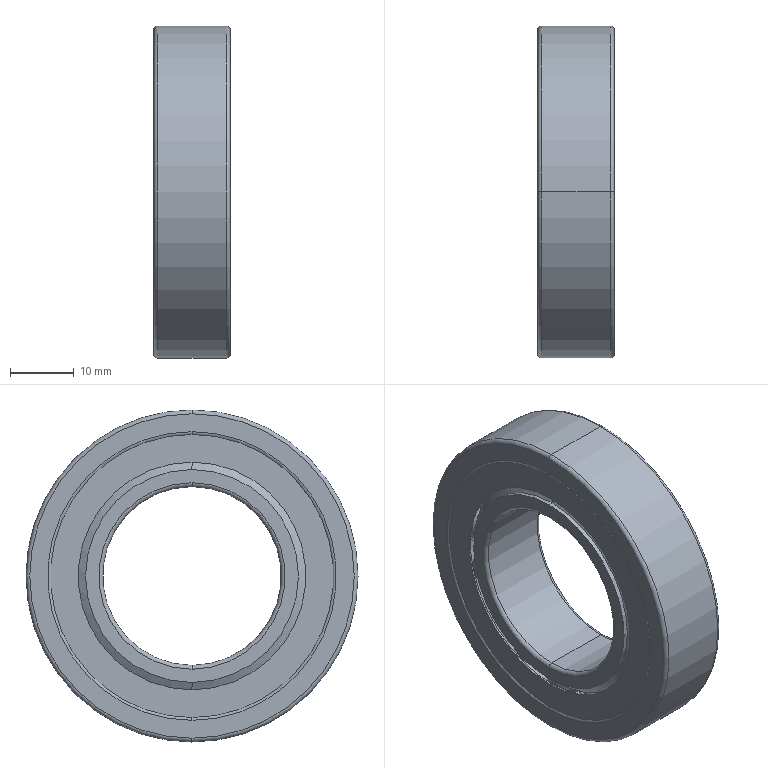Part | SolidWorks | features Revolution 5, CirPattern 2, RefAxis 1, RevCut 1 | 19 solids | 222 faces | box 12 x 52 x 52 mm | volume 13563 mm3 | cylinder 82 | sphere 72 | plane 42 | torus 22 | cone 4 | commonest cylinder face diameters 38.8 x33 41.2 x33 33.333 x4 36 x4 44 x4 28 x2